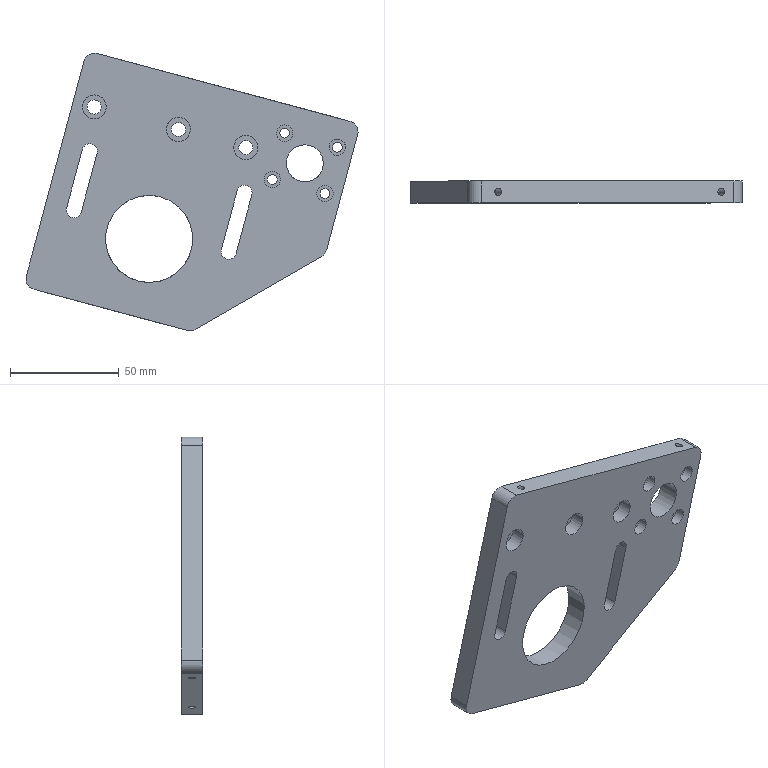Part | 1 solid | 51 faces | box 152.311 x 10 x 127.359 mm | volume 109635 mm3 | cylinder 29 | plane 22 | commonest cylinder face diameters 10 x5 3.3 x4 4.5 x4 7 x4 7.5 x4 6.5 x3
STEP:
#1=CARTESIAN_POINT('',(554.778,-302.903,7.909));
#2=VERTEX_POINT('',#1);
#3=CARTESIAN_POINT('',(554.778,-302.903,-0.5914));
#4=DIRECTION('',(0.,1.,0.));
#5=DIRECTION('',(0.,0.,1.));
#6=AXIS2_PLACEMENT_3D('',#3,#4,#5);
#7=CIRCLE('',#6,8.5);
#8=EDGE_CURVE('',#2,#2,#7,.T.);
#9=ORIENTED_EDGE('',*,*,#8,.T.);
#10=EDGE_LOOP('',(#9));
#11=FACE_BOUND('',#10,.T.);
#12=CARTESIAN_POINT('',(539.857,-302.903,-4.231));
#13=VERTEX_POINT('',#12);
#14=CARTESIAN_POINT('',(539.857,-302.903,-7.981));
#15=DIRECTION('',(0.,1.,0.));
#16=DIRECTION('',(0.,0.,1.));
#17=AXIS2_PLACEMENT_3D('',#14,#15,#16);
#18=CIRCLE('',#17,3.75);
#19=EDGE_CURVE('',#13,#13,#18,.T.);
#20=ORIENTED_EDGE('',*,*,#19,.T.);
#21=EDGE_LOOP('',(#20));
#22=FACE_BOUND('',#21,.T.);
#23=CARTESIAN_POINT('',(527.732,-302.903,12.156));
#24=VERTEX_POINT('',#23);
#25=CARTESIAN_POINT('',(527.732,-302.903,6.656));
#26=DIRECTION('',(0.,1.,0.));
#27=DIRECTION('',(0.,0.,1.));
#28=AXIS2_PLACEMENT_3D('',#25,#26,#27);
#29=CIRCLE('',#28,5.5);
#30=EDGE_CURVE('',#24,#24,#29,.T.);
#31=ORIENTED_EDGE('',*,*,#30,.T.);
#32=EDGE_LOOP('',(#31));
#33=FACE_BOUND('',#32,.T.);
#34=CARTESIAN_POINT('',(530.486,-302.903,-15.015));
#35=VERTEX_POINT('',#34);
#36=CARTESIAN_POINT('',(523.239,-302.903,-42.061));
#37=VERTEX_POINT('',#36);
#38=CARTESIAN_POINT('',(542.399,-302.903,29.442));
#39=DIRECTION('',(-0.2588,0.,-0.9659));
#40=VECTOR('',#39,1000.);
#41=LINE('',#38,#40);
#42=EDGE_CURVE('',#35,#37,#41,.T.);
#43=ORIENTED_EDGE('',*,*,#42,.T.);
#44=CARTESIAN_POINT('',(516.478,-302.903,-40.249));
#45=VERTEX_POINT('',#44);
#46=CARTESIAN_POINT('',(519.859,-302.903,-41.155));
#47=DIRECTION('',(0.,1.,0.));
#48=DIRECTION('',(0.,0.,1.));
#49=AXIS2_PLACEMENT_3D('',#46,#47,#48);
#50=CIRCLE('',#49,3.5);
#51=EDGE_CURVE('',#37,#45,#50,.T.);
#52=ORIENTED_EDGE('',*,*,#51,.T.);
#53=CARTESIAN_POINT('',(523.725,-302.903,-13.203));
#54=VERTEX_POINT('',#53);
#55=CARTESIAN_POINT('',(535.637,-302.903,31.254));
#56=DIRECTION('',(0.2588,0.,0.9659));
#57=VECTOR('',#56,1000.);
#58=LINE('',#55,#57);
#59=EDGE_CURVE('',#45,#54,#58,.T.);
#60=ORIENTED_EDGE('',*,*,#59,.T.);
#61=CARTESIAN_POINT('',(527.106,-302.903,-14.109));
#62=DIRECTION('',(0.,1.,0.));
#63=DIRECTION('',(0.,0.,1.));
#64=AXIS2_PLACEMENT_3D('',#61,#62,#63);
#65=CIRCLE('',#64,3.5);
#66=EDGE_CURVE('',#54,#35,#65,.T.);
#67=ORIENTED_EDGE('',*,*,#66,.T.);
#68=EDGE_LOOP('',(#43,#52,#60,#67));
#69=FACE_BOUND('',#68,.T.);
#70=CARTESIAN_POINT('',(562.508,-302.903,-43.357));
#71=VERTEX_POINT('',#70);
#72=CARTESIAN_POINT('',(564.838,-302.903,-40.321));
#73=VERTEX_POINT('',#72);
#74=CARTESIAN_POINT('',(560.008,-302.903,-39.027));
#75=DIRECTION('',(0.,1.,0.));
#76=DIRECTION('',(0.,0.,1.));
#77=AXIS2_PLACEMENT_3D('',#74,#75,#76);
#78=CIRCLE('',#77,5.);
#79=EDGE_CURVE('',#71,#73,#78,.F.);
#80=ORIENTED_EDGE('',*,*,#79,.T.);
#81=CARTESIAN_POINT('',(579.014,-302.903,12.585));
#82=VERTEX_POINT('',#81);
#83=CARTESIAN_POINT('',(572.802,-302.903,-10.597));
#84=DIRECTION('',(0.2588,0.,0.9659));
#85=VECTOR('',#84,1000.);
#86=LINE('',#83,#85);
#87=EDGE_CURVE('',#73,#82,#86,.T.);
#88=ORIENTED_EDGE('',*,*,#87,.T.);
#89=CARTESIAN_POINT('',(575.478,-302.903,18.709));
#90=VERTEX_POINT('',#89);
#91=CARTESIAN_POINT('',(574.184,-302.903,13.879));
#92=DIRECTION('',(0.,1.,0.));
#93=DIRECTION('',(0.,0.,1.));
#94=AXIS2_PLACEMENT_3D('',#91,#92,#93);
#95=CIRCLE('',#94,5.);
#96=EDGE_CURVE('',#82,#90,#95,.F.);
#97=ORIENTED_EDGE('',*,*,#96,.T.);
#98=CARTESIAN_POINT('',(459.567,-302.903,49.767));
#99=VERTEX_POINT('',#98);
#100=CARTESIAN_POINT('',(344.622,-302.903,80.566));
#101=DIRECTION('',(-0.9659,0.,0.2588));
#102=VECTOR('',#101,1000.);
#103=LINE('',#100,#102);
#104=EDGE_CURVE('',#90,#99,#103,.T.);
#105=ORIENTED_EDGE('',*,*,#104,.T.);
#106=CARTESIAN_POINT('',(453.443,-302.903,46.231));
#107=VERTEX_POINT('',#106);
#108=CARTESIAN_POINT('',(458.273,-302.903,44.937));
#109=DIRECTION('',(0.,1.,0.));
#110=DIRECTION('',(0.,0.,1.));
#111=AXIS2_PLACEMENT_3D('',#108,#109,#110);
#112=CIRCLE('',#111,5.);
#113=EDGE_CURVE('',#99,#107,#112,.F.);
#114=ORIENTED_EDGE('',*,*,#113,.T.);
#115=CARTESIAN_POINT('',(427.044,-302.903,-52.293));
#116=VERTEX_POINT('',#115);
#117=CARTESIAN_POINT('',(425.529,-302.903,-57.947));
#118=DIRECTION('',(-0.2588,0.,-0.9659));
#119=VECTOR('',#118,1000.);
#120=LINE('',#117,#119);
#121=EDGE_CURVE('',#107,#116,#120,.T.);
#122=ORIENTED_EDGE('',*,*,#121,.T.);
#123=CARTESIAN_POINT('',(430.579,-302.903,-58.417));
#124=VERTEX_POINT('',#123);
#125=CARTESIAN_POINT('',(431.874,-302.903,-53.587));
#126=DIRECTION('',(0.,1.,0.));
#127=DIRECTION('',(0.,0.,1.));
#128=AXIS2_PLACEMENT_3D('',#125,#126,#127);
#129=CIRCLE('',#128,5.);
#130=EDGE_CURVE('',#116,#124,#129,.F.);
#131=ORIENTED_EDGE('',*,*,#130,.T.);
#132=CARTESIAN_POINT('',(500.872,-302.903,-77.252));
#133=VERTEX_POINT('',#132);
#134=CARTESIAN_POINT('',(300.037,-302.903,-23.438));
#135=DIRECTION('',(0.9659,0.,-0.2588));
#136=VECTOR('',#135,1000.);
#137=LINE('',#134,#136);
#138=EDGE_CURVE('',#124,#133,#137,.T.);
#139=ORIENTED_EDGE('',*,*,#138,.T.);
#140=CARTESIAN_POINT('',(504.666,-302.903,-76.752));
#141=VERTEX_POINT('',#140);
#142=CARTESIAN_POINT('',(502.166,-302.903,-72.422));
#143=DIRECTION('',(0.,1.,0.));
#144=DIRECTION('',(0.,0.,1.));
#145=AXIS2_PLACEMENT_3D('',#142,#143,#144);
#146=CIRCLE('',#145,5.);
#147=EDGE_CURVE('',#133,#141,#146,.F.);
#148=ORIENTED_EDGE('',*,*,#147,.T.);
#149=CARTESIAN_POINT('',(528.994,-302.903,-62.706));
#150=DIRECTION('',(-0.866,0.,-0.5));
#151=VECTOR('',#150,1000.);
#152=LINE('',#149,#151);
#153=EDGE_CURVE('',#71,#141,#152,.T.);
#154=ORIENTED_EDGE('',*,*,#153,.F.);
#155=EDGE_LOOP('',(#80,#88,#97,#105,#114,#122,#131,#139,#148,#154));
#156=FACE_BOUND('',#155,.T.);
#157=CARTESIAN_POINT('',(452.206,-302.903,-23.027));
#158=VERTEX_POINT('',#157);
#159=CARTESIAN_POINT('',(445.445,-302.903,-21.216));
#160=VERTEX_POINT('',#159);
#161=CARTESIAN_POINT('',(448.826,-302.903,-22.122));
#162=DIRECTION('',(0.,1.,0.));
#163=DIRECTION('',(0.,0.,1.));
#164=AXIS2_PLACEMENT_3D('',#161,#162,#163);
#165=CIRCLE('',#164,3.5);
#166=EDGE_CURVE('',#158,#160,#165,.T.);
#167=ORIENTED_EDGE('',*,*,#166,.T.);
#168=CARTESIAN_POINT('',(452.692,-302.903,5.83));
#169=VERTEX_POINT('',#168);
#170=CARTESIAN_POINT('',(464.604,-302.903,50.287));
#171=DIRECTION('',(0.2588,0.,0.9659));
#172=VECTOR('',#171,1000.);
#173=LINE('',#170,#172);
#174=EDGE_CURVE('',#160,#169,#173,.T.);
#175=ORIENTED_EDGE('',*,*,#174,.T.);
#176=CARTESIAN_POINT('',(459.453,-302.903,4.018));
#177=VERTEX_POINT('',#176);
#178=CARTESIAN_POINT('',(456.072,-302.903,4.924));
#179=DIRECTION('',(0.,1.,0.));
#180=DIRECTION('',(0.,0.,1.));
#181=AXIS2_PLACEMENT_3D('',#178,#179,#180);
#182=CIRCLE('',#181,3.5);
#183=EDGE_CURVE('',#169,#177,#182,.T.);
#184=ORIENTED_EDGE('',*,*,#183,.T.);
#185=CARTESIAN_POINT('',(471.365,-302.903,48.476));
#186=DIRECTION('',(-0.2588,0.,-0.9659));
#187=VECTOR('',#186,1000.);
#188=LINE('',#185,#187);
#189=EDGE_CURVE('',#177,#158,#188,.T.);
#190=ORIENTED_EDGE('',*,*,#189,.T.);
#191=EDGE_LOOP('',(#167,#175,#184,#190));
#192=FACE_BOUND('',#191,.T.);
#193=CARTESIAN_POINT('',(569.699,-302.903,10.549));
#194=VERTEX_POINT('',#193);
#195=CARTESIAN_POINT('',(569.699,-302.903,6.799));
#196=DIRECTION('',(0.,1.,0.));
#197=DIRECTION('',(0.,0.,1.));
#198=AXIS2_PLACEMENT_3D('',#195,#196,#197);
#199=CIRCLE('',#198,3.75);
#200=EDGE_CURVE('',#194,#194,#199,.T.);
#201=ORIENTED_EDGE('',*,*,#200,.T.);
#202=EDGE_LOOP('',(#201));
#203=FACE_BOUND('',#202,.T.);
#204=CARTESIAN_POINT('',(458.185,-302.903,30.791));
#205=VERTEX_POINT('',#204);
#206=CARTESIAN_POINT('',(458.185,-302.903,25.291));
#207=DIRECTION('',(0.,1.,0.));
#208=DIRECTION('',(0.,0.,1.));
#209=AXIS2_PLACEMENT_3D('',#206,#207,#208);
#210=CIRCLE('',#209,5.5);
#211=EDGE_CURVE('',#205,#205,#210,.T.);
#212=ORIENTED_EDGE('',*,*,#211,.T.);
#213=EDGE_LOOP('',(#212));
#214=FACE_BOUND('',#213,.T.);
#215=CARTESIAN_POINT('',(496.822,-302.903,20.438));
#216=VERTEX_POINT('',#215);
#217=CARTESIAN_POINT('',(496.822,-302.903,14.938));
#218=DIRECTION('',(0.,1.,0.));
#219=DIRECTION('',(0.,0.,1.));
#220=AXIS2_PLACEMENT_3D('',#217,#218,#219);
#221=CIRCLE('',#220,5.5);
#222=EDGE_CURVE('',#216,#216,#221,.T.);
#223=ORIENTED_EDGE('',*,*,#222,.T.);
#224=EDGE_LOOP('',(#223));
#225=FACE_BOUND('',#224,.T.);
#226=CARTESIAN_POINT('',(564.005,-302.903,-10.702));
#227=VERTEX_POINT('',#226);
#228=CARTESIAN_POINT('',(564.005,-302.903,-14.452));
#229=DIRECTION('',(0.,1.,0.));
#230=DIRECTION('',(0.,0.,1.));
#231=AXIS2_PLACEMENT_3D('',#228,#229,#230);
#232=CIRCLE('',#231,3.75);
#233=EDGE_CURVE('',#227,#227,#232,.T.);
#234=ORIENTED_EDGE('',*,*,#233,.T.);
#235=EDGE_LOOP('',(#234));
#236=FACE_BOUND('',#235,.T.);
#237=CARTESIAN_POINT('',(545.551,-302.903,17.019));
#238=VERTEX_POINT('',#237);
#239=CARTESIAN_POINT('',(545.551,-302.903,13.269));
#240=DIRECTION('',(0.,1.,0.));
#241=DIRECTION('',(0.,0.,1.));
#242=AXIS2_PLACEMENT_3D('',#239,#240,#241);
#243=CIRCLE('',#242,3.75);
#244=EDGE_CURVE('',#238,#238,#243,.T.);
#245=ORIENTED_EDGE('',*,*,#244,.T.);
#246=EDGE_LOOP('',(#245));
#247=FACE_BOUND('',#246,.T.);
#248=CARTESIAN_POINT('',(483.367,-302.903,-15.279));
#249=VERTEX_POINT('',#248);
#250=CARTESIAN_POINT('',(483.367,-302.903,-35.279));
#251=DIRECTION('',(0.,1.,0.));
#252=DIRECTION('',(0.,0.,1.));
#253=AXIS2_PLACEMENT_3D('',#250,#251,#252);
#254=CIRCLE('',#253,20.);
#255=EDGE_CURVE('',#249,#249,#254,.T.);
#256=ORIENTED_EDGE('',*,*,#255,.T.);
#257=EDGE_LOOP('',(#256));
#258=FACE_BOUND('',#257,.T.);
#259=CARTESIAN_POINT('',(599.269,-302.903,14.204));
#260=DIRECTION('',(0.,1.,0.));
#261=DIRECTION('',(0.7196,0.,-0.6944));
#262=AXIS2_PLACEMENT_3D('',#259,#260,#261);
#263=PLANE('',#262);
#264=ADVANCED_FACE('',(#11,#22,#33,#69,#156,#192,#203,#214,#225,#236,#247,#258),#263,.F.);
#265=CARTESIAN_POINT('',(492.717,-297.903,-64.714));
#266=VERTEX_POINT('',#265);
#267=CARTESIAN_POINT('',(491.123,-297.903,-64.287));
#268=DIRECTION('',(0.2588,0.,0.9659));
#269=DIRECTION('',(0.9659,0.,-0.2588));
#270=AXIS2_PLACEMENT_3D('',#267,#268,#269);
#271=CIRCLE('',#270,1.65);
#272=EDGE_CURVE('',#266,#266,#271,.T.);
#273=ORIENTED_EDGE('',*,*,#272,.T.);
#274=EDGE_LOOP('',(#273));
#275=FACE_BOUND('',#274,.T.);
#276=CARTESIAN_POINT('',(490.129,-297.903,-74.373));
#277=VERTEX_POINT('',#276);
#278=CARTESIAN_POINT('',(488.535,-297.903,-73.946));
#279=DIRECTION('',(0.2588,0.,0.9659));
#280=DIRECTION('',(0.9659,0.,-0.2588));
#281=AXIS2_PLACEMENT_3D('',#278,#279,#280);
#282=CIRCLE('',#281,1.65);
#283=EDGE_CURVE('',#277,#277,#282,.T.);
#284=ORIENTED_EDGE('',*,*,#283,.F.);
#285=EDGE_LOOP('',(#284));
#286=FACE_BOUND('',#285,.T.);
#287=CARTESIAN_POINT('',(489.829,-297.903,-69.116));
#288=DIRECTION('',(-0.2588,0.,-0.9659));
#289=DIRECTION('',(0.,1.,0.));
#290=AXIS2_PLACEMENT_3D('',#287,#288,#289);
#291=CYLINDRICAL_SURFACE('',#290,1.65);
#292=ADVANCED_FACE('',(#275,#286),#291,.F.);
#293=ORIENTED_EDGE('',*,*,#272,.F.);
#294=EDGE_LOOP('',(#293));
#295=FACE_BOUND('',#294,.T.);
#296=CARTESIAN_POINT('',(442.827,-297.903,-51.346));
#297=DIRECTION('',(0.2588,0.,0.9659));
#298=DIRECTION('',(-0.9659,0.,0.2588));
#299=AXIS2_PLACEMENT_3D('',#296,#297,#298);
#300=PLANE('',#299);
#301=ADVANCED_FACE('',(#295),#300,.F.);
#302=CARTESIAN_POINT('',(568.302,-298.98,10.279));
#303=VERTEX_POINT('',#302);
#304=CARTESIAN_POINT('',(568.669,-298.403,10.405));
#305=VERTEX_POINT('',#304);
#306=CARTESIAN_POINT('',(568.302,-298.98,10.279));
#307=CARTESIAN_POINT('',(568.462,-298.819,10.343));
#308=CARTESIAN_POINT('',(568.591,-298.624,10.382));
#309=CARTESIAN_POINT('',(568.669,-298.403,10.405));
#310=B_SPLINE_CURVE_WITH_KNOTS('',3,(#306,#307,#308,#309),.UNSPECIFIED.,.F.,.F.,(4,4),(0.,0.0006972),.UNSPECIFIED.);
#311=EDGE_CURVE('',#303,#305,#310,.T.);
#312=ORIENTED_EDGE('',*,*,#311,.F.);
#313=CARTESIAN_POINT('',(568.613,-298.403,10.195));
#314=VERTEX_POINT('',#313);
#315=CARTESIAN_POINT('',(567.095,-297.903,10.602));
#316=DIRECTION('',(-0.2588,0.,-0.9659));
#317=DIRECTION('',(-0.9659,0.,0.2588));
#318=AXIS2_PLACEMENT_3D('',#315,#316,#317);
#319=CIRCLE('',#318,1.65);
#320=EDGE_CURVE('',#303,#314,#319,.T.);
#321=ORIENTED_EDGE('',*,*,#320,.T.);
#322=CARTESIAN_POINT('',(569.907,-298.403,15.025));
#323=DIRECTION('',(-0.2588,0.,-0.9659));
#324=VECTOR('',#323,1000.);
#325=LINE('',#322,#324);
#326=EDGE_CURVE('',#305,#314,#325,.T.);
#327=ORIENTED_EDGE('',*,*,#326,.F.);
#328=EDGE_LOOP('',(#312,#321,#327));
#329=FACE_BOUND('',#328,.T.);
#330=CARTESIAN_POINT('',(568.089,-297.903,20.689));
#331=VERTEX_POINT('',#330);
#332=CARTESIAN_POINT('',(569.683,-297.903,20.261));
#333=DIRECTION('',(-0.2588,0.,-0.9659));
#334=DIRECTION('',(-0.9659,0.,0.2588));
#335=AXIS2_PLACEMENT_3D('',#332,#333,#334);
#336=CIRCLE('',#335,1.65);
#337=EDGE_CURVE('',#331,#331,#336,.T.);
#338=ORIENTED_EDGE('',*,*,#337,.F.);
#339=EDGE_LOOP('',(#338));
#340=FACE_BOUND('',#339,.T.);
#341=CARTESIAN_POINT('',(568.389,-297.903,15.432));
#342=DIRECTION('',(0.2588,0.,0.9659));
#343=DIRECTION('',(0.,1.,0.));
#344=AXIS2_PLACEMENT_3D('',#341,#342,#343);
#345=CYLINDRICAL_SURFACE('',#344,1.65);
#346=ADVANCED_FACE('',(#329,#340),#345,.F.);
#347=ORIENTED_EDGE('',*,*,#320,.F.);
#348=CARTESIAN_POINT('',(568.302,-298.403,10.279));
#349=VERTEX_POINT('',#348);
#350=CARTESIAN_POINT('',(568.302,-302.903,10.279));
#351=DIRECTION('',(0.,-1.,0.));
#352=VECTOR('',#351,1000.);
#353=LINE('',#350,#352);
#354=EDGE_CURVE('',#349,#303,#353,.T.);
#355=ORIENTED_EDGE('',*,*,#354,.F.);
#356=CARTESIAN_POINT('',(570.475,-298.403,9.696));
#357=DIRECTION('',(-0.9659,0.,0.2588));
#358=VECTOR('',#357,1000.);
#359=LINE('',#356,#358);
#360=EDGE_CURVE('',#314,#349,#359,.T.);
#361=ORIENTED_EDGE('',*,*,#360,.F.);
#362=EDGE_LOOP('',(#347,#355,#361));
#363=FACE_BOUND('',#362,.T.);
#364=CARTESIAN_POINT('',(466.638,-297.903,37.519));
#365=DIRECTION('',(-0.2588,0.,-0.9659));
#366=DIRECTION('',(-0.9659,0.,0.2588));
#367=AXIS2_PLACEMENT_3D('',#364,#365,#366);
#368=PLANE('',#367);
#369=ADVANCED_FACE('',(#363),#368,.F.);
#370=CARTESIAN_POINT('',(442.489,-297.903,-51.255));
#371=VERTEX_POINT('',#370);
#372=CARTESIAN_POINT('',(440.895,-297.903,-50.828));
#373=DIRECTION('',(0.2588,0.,0.9659));
#374=DIRECTION('',(0.9659,0.,-0.2588));
#375=AXIS2_PLACEMENT_3D('',#372,#373,#374);
#376=CIRCLE('',#375,1.65);
#377=EDGE_CURVE('',#371,#371,#376,.T.);
#378=ORIENTED_EDGE('',*,*,#377,.T.);
#379=EDGE_LOOP('',(#378));
#380=FACE_BOUND('',#379,.T.);
#381=CARTESIAN_POINT('',(436.713,-297.903,-60.06));
#382=VERTEX_POINT('',#381);
#383=CARTESIAN_POINT('',(438.307,-297.903,-60.487));
#384=DIRECTION('',(0.2588,0.,0.9659));
#385=DIRECTION('',(-0.9659,0.,0.2588));
#386=AXIS2_PLACEMENT_3D('',#383,#384,#385);
#387=CIRCLE('',#386,1.65);
#388=EDGE_CURVE('',#382,#382,#387,.T.);
#389=ORIENTED_EDGE('',*,*,#388,.F.);
#390=EDGE_LOOP('',(#389));
#391=FACE_BOUND('',#390,.T.);
#392=CARTESIAN_POINT('',(466.,-297.903,42.867));
#393=DIRECTION('',(0.2588,0.,0.9659));
#394=DIRECTION('',(0.,1.,0.));
#395=AXIS2_PLACEMENT_3D('',#392,#393,#394);
#396=CYLINDRICAL_SURFACE('',#395,1.65);
#397=ADVANCED_FACE('',(#380,#391),#396,.F.);
#398=ORIENTED_EDGE('',*,*,#377,.F.);
#399=EDGE_LOOP('',(#398));
#400=FACE_BOUND('',#399,.T.);
#401=CARTESIAN_POINT('',(442.827,-297.903,-51.346));
#402=DIRECTION('',(0.2588,0.,0.9659));
#403=DIRECTION('',(-0.9659,0.,0.2588));
#404=AXIS2_PLACEMENT_3D('',#401,#402,#403);
#405=PLANE('',#404);
#406=ADVANCED_FACE('',(#400),#405,.F.);
#407=CARTESIAN_POINT('',(463.113,-297.903,38.464));
#408=VERTEX_POINT('',#407);
#409=CARTESIAN_POINT('',(464.706,-297.903,38.037));
#410=DIRECTION('',(-0.2588,0.,-0.9659));
#411=DIRECTION('',(-0.9659,0.,0.2588));
#412=AXIS2_PLACEMENT_3D('',#409,#410,#411);
#413=CIRCLE('',#412,1.65);
#414=EDGE_CURVE('',#408,#408,#413,.T.);
#415=ORIENTED_EDGE('',*,*,#414,.T.);
#416=EDGE_LOOP('',(#415));
#417=FACE_BOUND('',#416,.T.);
#418=CARTESIAN_POINT('',(468.888,-297.903,47.269));
#419=VERTEX_POINT('',#418);
#420=CARTESIAN_POINT('',(467.295,-297.903,47.696));
#421=DIRECTION('',(-0.2588,0.,-0.9659));
#422=DIRECTION('',(0.9659,0.,-0.2588));
#423=AXIS2_PLACEMENT_3D('',#420,#421,#422);
#424=CIRCLE('',#423,1.65);
#425=EDGE_CURVE('',#419,#419,#424,.T.);
#426=ORIENTED_EDGE('',*,*,#425,.F.);
#427=EDGE_LOOP('',(#426));
#428=FACE_BOUND('',#427,.T.);
#429=CARTESIAN_POINT('',(466.,-297.903,42.867));
#430=DIRECTION('',(0.2588,0.,0.9659));
#431=DIRECTION('',(0.,1.,0.));
#432=AXIS2_PLACEMENT_3D('',#429,#430,#431);
#433=CYLINDRICAL_SURFACE('',#432,1.65);
#434=ADVANCED_FACE('',(#417,#428),#433,.F.);
#435=ORIENTED_EDGE('',*,*,#414,.F.);
#436=EDGE_LOOP('',(#435));
#437=FACE_BOUND('',#436,.T.);
#438=CARTESIAN_POINT('',(466.638,-297.903,37.519));
#439=DIRECTION('',(-0.2588,0.,-0.9659));
#440=DIRECTION('',(-0.9659,0.,0.2588));
#441=AXIS2_PLACEMENT_3D('',#438,#439,#440);
#442=PLANE('',#441);
#443=ADVANCED_FACE('',(#437),#442,.F.);
#444=CARTESIAN_POINT('',(564.005,-298.403,-10.702));
#445=VERTEX_POINT('',#444);
#446=CARTESIAN_POINT('',(564.005,-298.403,-14.452));
#447=DIRECTION('',(0.,-1.,0.));
#448=DIRECTION('',(0.,0.,1.));
#449=AXIS2_PLACEMENT_3D('',#446,#447,#448);
#450=CIRCLE('',#449,3.75);
#451=EDGE_CURVE('',#445,#445,#450,.T.);
#452=ORIENTED_EDGE('',*,*,#451,.F.);
#453=EDGE_LOOP('',(#452));
#454=FACE_BOUND('',#453,.T.);
#455=ORIENTED_EDGE('',*,*,#233,.F.);
#456=EDGE_LOOP('',(#455));
#457=FACE_BOUND('',#456,.T.);
#458=CARTESIAN_POINT('',(564.005,-302.903,-14.452));
#459=DIRECTION('',(0.,1.,0.));
#460=DIRECTION('',(-0.9659,0.,0.2588));
#461=AXIS2_PLACEMENT_3D('',#458,#459,#460);
#462=CYLINDRICAL_SURFACE('',#461,3.75);
#463=ADVANCED_FACE('',(#454,#457),#462,.F.);
#464=ORIENTED_EDGE('',*,*,#451,.T.);
#465=EDGE_LOOP('',(#464));
#466=FACE_BOUND('',#465,.T.);
#467=CARTESIAN_POINT('',(564.005,-298.403,-12.202));
#468=VERTEX_POINT('',#467);
#469=CARTESIAN_POINT('',(564.005,-298.403,-14.452));
#470=DIRECTION('',(0.,-1.,0.));
#471=DIRECTION('',(0.,0.,1.));
#472=AXIS2_PLACEMENT_3D('',#469,#470,#471);
#473=CIRCLE('',#472,2.25);
#474=EDGE_CURVE('',#468,#468,#473,.T.);
#475=ORIENTED_EDGE('',*,*,#474,.F.);
#476=EDGE_LOOP('',(#475));
#477=FACE_BOUND('',#476,.T.);
#478=CARTESIAN_POINT('',(569.699,-298.403,6.799));
#479=DIRECTION('',(0.,1.,0.));
#480=DIRECTION('',(-0.9659,0.,0.2588));
#481=AXIS2_PLACEMENT_3D('',#478,#479,#480);
#482=PLANE('',#481);
#483=ADVANCED_FACE('',(#466,#477),#482,.F.);
#484=CARTESIAN_POINT('',(564.587,-292.903,-12.278));
#485=VERTEX_POINT('',#484);
#486=CARTESIAN_POINT('',(564.005,-292.903,-14.452));
#487=DIRECTION('',(0.,1.,0.));
#488=DIRECTION('',(0.2588,0.,0.9659));
#489=AXIS2_PLACEMENT_3D('',#486,#487,#488);
#490=CIRCLE('',#489,2.25);
#491=EDGE_CURVE('',#485,#485,#490,.T.);
#492=ORIENTED_EDGE('',*,*,#491,.T.);
#493=EDGE_LOOP('',(#492));
#494=FACE_BOUND('',#493,.T.);
#495=ORIENTED_EDGE('',*,*,#474,.T.);
#496=EDGE_LOOP('',(#495));
#497=FACE_BOUND('',#496,.T.);
#498=CARTESIAN_POINT('',(564.005,-232.903,-14.452));
#499=DIRECTION('',(0.,1.,0.));
#500=DIRECTION('',(-0.9659,0.,0.2588));
#501=AXIS2_PLACEMENT_3D('',#498,#499,#500);
#502=CYLINDRICAL_SURFACE('',#501,2.25);
#503=ADVANCED_FACE('',(#494,#497),#502,.F.);
#504=CARTESIAN_POINT('',(569.699,-298.403,6.799));
#505=DIRECTION('',(0.,1.,0.));
#506=DIRECTION('',(-0.9659,0.,0.2588));
#507=AXIS2_PLACEMENT_3D('',#504,#505,#506);
#508=CIRCLE('',#507,3.75);
#509=EDGE_CURVE('',#305,#349,#508,.T.);
#510=ORIENTED_EDGE('',*,*,#509,.T.);
#511=ORIENTED_EDGE('',*,*,#354,.T.);
#512=ORIENTED_EDGE('',*,*,#311,.T.);
#513=EDGE_LOOP('',(#510,#511,#512));
#514=FACE_BOUND('',#513,.T.);
#515=ORIENTED_EDGE('',*,*,#200,.F.);
#516=EDGE_LOOP('',(#515));
#517=FACE_BOUND('',#516,.T.);
#518=CARTESIAN_POINT('',(569.699,-302.903,6.799));
#519=DIRECTION('',(0.,1.,0.));
#520=DIRECTION('',(-0.9659,0.,0.2588));
#521=AXIS2_PLACEMENT_3D('',#518,#519,#520);
#522=CYLINDRICAL_SURFACE('',#521,3.75);
#523=ADVANCED_FACE('',(#514,#517),#522,.F.);
#524=ORIENTED_EDGE('',*,*,#326,.T.);
#525=ORIENTED_EDGE('',*,*,#360,.T.);
#526=ORIENTED_EDGE('',*,*,#509,.F.);
#527=EDGE_LOOP('',(#524,#525,#526));
#528=FACE_BOUND('',#527,.T.);
#529=CARTESIAN_POINT('',(567.525,-298.403,7.381));
#530=VERTEX_POINT('',#529);
#531=CARTESIAN_POINT('',(569.699,-298.403,6.799));
#532=DIRECTION('',(0.,1.,0.));
#533=DIRECTION('',(-0.9659,0.,0.2588));
#534=AXIS2_PLACEMENT_3D('',#531,#532,#533);
#535=CIRCLE('',#534,2.25);
#536=EDGE_CURVE('',#530,#530,#535,.T.);
#537=ORIENTED_EDGE('',*,*,#536,.T.);
#538=EDGE_LOOP('',(#537));
#539=FACE_BOUND('',#538,.T.);
#540=CARTESIAN_POINT('',(569.699,-298.403,6.799));
#541=DIRECTION('',(0.,1.,0.));
#542=DIRECTION('',(-0.9659,0.,0.2588));
#543=AXIS2_PLACEMENT_3D('',#540,#541,#542);
#544=PLANE('',#543);
#545=ADVANCED_FACE('',(#528,#539),#544,.F.);
#546=CARTESIAN_POINT('',(570.281,-292.903,8.972));
#547=VERTEX_POINT('',#546);
#548=CARTESIAN_POINT('',(569.699,-292.903,6.799));
#549=DIRECTION('',(0.,-1.,0.));
#550=DIRECTION('',(0.2588,0.,0.9659));
#551=AXIS2_PLACEMENT_3D('',#548,#549,#550);
#552=CIRCLE('',#551,2.25);
#553=EDGE_CURVE('',#547,#547,#552,.T.);
#554=ORIENTED_EDGE('',*,*,#553,.F.);
#555=EDGE_LOOP('',(#554));
#556=FACE_BOUND('',#555,.T.);
#557=ORIENTED_EDGE('',*,*,#536,.F.);
#558=EDGE_LOOP('',(#557));
#559=FACE_BOUND('',#558,.T.);
#560=CARTESIAN_POINT('',(569.699,-232.903,6.799));
#561=DIRECTION('',(0.,1.,0.));
#562=DIRECTION('',(-0.9659,0.,0.2588));
#563=AXIS2_PLACEMENT_3D('',#560,#561,#562);
#564=CYLINDRICAL_SURFACE('',#563,2.25);
#565=ADVANCED_FACE('',(#556,#559),#564,.F.);
#566=CARTESIAN_POINT('',(539.857,-298.403,-4.231));
#567=VERTEX_POINT('',#566);
#568=CARTESIAN_POINT('',(539.857,-298.403,-7.981));
#569=DIRECTION('',(0.,1.,0.));
#570=DIRECTION('',(0.,0.,1.));
#571=AXIS2_PLACEMENT_3D('',#568,#569,#570);
#572=CIRCLE('',#571,3.75);
#573=EDGE_CURVE('',#567,#567,#572,.T.);
#574=ORIENTED_EDGE('',*,*,#573,.T.);
#575=EDGE_LOOP('',(#574));
#576=FACE_BOUND('',#575,.T.);
#577=ORIENTED_EDGE('',*,*,#19,.F.);
#578=EDGE_LOOP('',(#577));
#579=FACE_BOUND('',#578,.T.);
#580=CARTESIAN_POINT('',(539.857,-302.903,-7.981));
#581=DIRECTION('',(0.,1.,0.));
#582=DIRECTION('',(-0.9659,0.,0.2588));
#583=AXIS2_PLACEMENT_3D('',#580,#581,#582);
#584=CYLINDRICAL_SURFACE('',#583,3.75);
#585=ADVANCED_FACE('',(#576,#579),#584,.F.);
#586=ORIENTED_EDGE('',*,*,#573,.F.);
#587=EDGE_LOOP('',(#586));
#588=FACE_BOUND('',#587,.T.);
#589=CARTESIAN_POINT('',(539.857,-298.403,-5.731));
#590=VERTEX_POINT('',#589);
#591=CARTESIAN_POINT('',(539.857,-298.403,-7.981));
#592=DIRECTION('',(0.,1.,0.));
#593=DIRECTION('',(0.,0.,1.));
#594=AXIS2_PLACEMENT_3D('',#591,#592,#593);
#595=CIRCLE('',#594,2.25);
#596=EDGE_CURVE('',#590,#590,#595,.T.);
#597=ORIENTED_EDGE('',*,*,#596,.T.);
#598=EDGE_LOOP('',(#597));
#599=FACE_BOUND('',#598,.T.);
#600=CARTESIAN_POINT('',(569.699,-298.403,6.799));
#601=DIRECTION('',(0.,1.,0.));
#602=DIRECTION('',(-0.9659,0.,0.2588));
#603=AXIS2_PLACEMENT_3D('',#600,#601,#602);
#604=PLANE('',#603);
#605=ADVANCED_FACE('',(#588,#599),#604,.F.);
#606=CARTESIAN_POINT('',(540.439,-292.903,-5.808));
#607=VERTEX_POINT('',#606);
#608=CARTESIAN_POINT('',(539.857,-292.903,-7.981));
#609=DIRECTION('',(0.,-1.,0.));
#610=DIRECTION('',(0.2588,0.,0.9659));
#611=AXIS2_PLACEMENT_3D('',#608,#609,#610);
#612=CIRCLE('',#611,2.25);
#613=EDGE_CURVE('',#607,#607,#612,.T.);
#614=ORIENTED_EDGE('',*,*,#613,.F.);
#615=EDGE_LOOP('',(#614));
#616=FACE_BOUND('',#615,.T.);
#617=ORIENTED_EDGE('',*,*,#596,.F.);
#618=EDGE_LOOP('',(#617));
#619=FACE_BOUND('',#618,.T.);
#620=CARTESIAN_POINT('',(539.857,-232.903,-7.981));
#621=DIRECTION('',(0.,1.,0.));
#622=DIRECTION('',(-0.9659,0.,0.2588));
#623=AXIS2_PLACEMENT_3D('',#620,#621,#622);
#624=CYLINDRICAL_SURFACE('',#623,2.25);
#625=ADVANCED_FACE('',(#616,#619),#624,.F.);
#626=CARTESIAN_POINT('',(545.551,-298.403,17.019));
#627=VERTEX_POINT('',#626);
#628=CARTESIAN_POINT('',(545.551,-298.403,13.269));
#629=DIRECTION('',(0.,-1.,0.));
#630=DIRECTION('',(0.,0.,1.));
#631=AXIS2_PLACEMENT_3D('',#628,#629,#630);
#632=CIRCLE('',#631,3.75);
#633=EDGE_CURVE('',#627,#627,#632,.T.);
#634=ORIENTED_EDGE('',*,*,#633,.F.);
#635=EDGE_LOOP('',(#634));
#636=FACE_BOUND('',#635,.T.);
#637=ORIENTED_EDGE('',*,*,#244,.F.);
#638=EDGE_LOOP('',(#637));
#639=FACE_BOUND('',#638,.T.);
#640=CARTESIAN_POINT('',(545.551,-302.903,13.269));
#641=DIRECTION('',(0.,1.,0.));
#642=DIRECTION('',(-0.9659,0.,0.2588));
#643=AXIS2_PLACEMENT_3D('',#640,#641,#642);
#644=CYLINDRICAL_SURFACE('',#643,3.75);
#645=ADVANCED_FACE('',(#636,#639),#644,.F.);
#646=ORIENTED_EDGE('',*,*,#633,.T.);
#647=EDGE_LOOP('',(#646));
#648=FACE_BOUND('',#647,.T.);
#649=CARTESIAN_POINT('',(545.551,-298.403,15.519));
#650=VERTEX_POINT('',#649);
#651=CARTESIAN_POINT('',(545.551,-298.403,13.269));
#652=DIRECTION('',(0.,-1.,0.));
#653=DIRECTION('',(0.,0.,1.));
#654=AXIS2_PLACEMENT_3D('',#651,#652,#653);
#655=CIRCLE('',#654,2.25);
#656=EDGE_CURVE('',#650,#650,#655,.T.);
#657=ORIENTED_EDGE('',*,*,#656,.F.);
#658=EDGE_LOOP('',(#657));
#659=FACE_BOUND('',#658,.T.);
#660=CARTESIAN_POINT('',(569.699,-298.403,6.799));
#661=DIRECTION('',(0.,1.,0.));
#662=DIRECTION('',(-0.9659,0.,0.2588));
#663=AXIS2_PLACEMENT_3D('',#660,#661,#662);
#664=PLANE('',#663);
#665=ADVANCED_FACE('',(#648,#659),#664,.F.);
#666=CARTESIAN_POINT('',(546.133,-292.903,15.442));
#667=VERTEX_POINT('',#666);
#668=CARTESIAN_POINT('',(545.551,-292.903,13.269));
#669=DIRECTION('',(0.,-1.,0.));
#670=DIRECTION('',(0.2588,0.,0.9659));
#671=AXIS2_PLACEMENT_3D('',#668,#669,#670);
#672=CIRCLE('',#671,2.25);
#673=EDGE_CURVE('',#667,#667,#672,.T.);
#674=ORIENTED_EDGE('',*,*,#673,.F.);
#675=EDGE_LOOP('',(#674));
#676=FACE_BOUND('',#675,.T.);
#677=ORIENTED_EDGE('',*,*,#656,.T.);
#678=EDGE_LOOP('',(#677));
#679=FACE_BOUND('',#678,.T.);
#680=CARTESIAN_POINT('',(545.551,-232.903,13.269));
#681=DIRECTION('',(0.,1.,0.));
#682=DIRECTION('',(-0.9659,0.,0.2588));
#683=AXIS2_PLACEMENT_3D('',#680,#681,#682);
#684=CYLINDRICAL_SURFACE('',#683,2.25);
#685=ADVANCED_FACE('',(#676,#679),#684,.F.);
#686=ORIENTED_EDGE('',*,*,#113,.F.);
#687=CARTESIAN_POINT('',(459.567,-292.903,49.767));
#688=VERTEX_POINT('',#687);
#689=CARTESIAN_POINT('',(459.567,-302.903,49.767));
#690=DIRECTION('',(0.,-1.,0.));
#691=VECTOR('',#690,1000.);
#692=LINE('',#689,#691);
#693=EDGE_CURVE('',#688,#99,#692,.T.);
#694=ORIENTED_EDGE('',*,*,#693,.F.);
#695=CARTESIAN_POINT('',(453.443,-292.903,46.231));
#696=VERTEX_POINT('',#695);
#697=CARTESIAN_POINT('',(458.273,-292.903,44.937));
#698=DIRECTION('',(0.,1.,0.));
#699=DIRECTION('',(0.2588,0.,0.9659));
#700=AXIS2_PLACEMENT_3D('',#697,#698,#699);
#701=CIRCLE('',#700,5.);
#702=EDGE_CURVE('',#696,#688,#701,.T.);
#703=ORIENTED_EDGE('',*,*,#702,.F.);
#704=CARTESIAN_POINT('',(453.443,-292.903,46.231));
#705=DIRECTION('',(0.,1.,0.));
#706=VECTOR('',#705,1000.);
#707=LINE('',#704,#706);
#708=EDGE_CURVE('',#107,#696,#707,.T.);
#709=ORIENTED_EDGE('',*,*,#708,.F.);
#710=EDGE_LOOP('',(#686,#694,#703,#709));
#711=FACE_BOUND('',#710,.T.);
#712=CARTESIAN_POINT('',(458.273,-270.003,44.937));
#713=DIRECTION('',(0.,1.,0.));
#714=DIRECTION('',(-0.9659,0.,0.2588));
#715=AXIS2_PLACEMENT_3D('',#712,#713,#714);
#716=CYLINDRICAL_SURFACE('',#715,5.);
#717=ADVANCED_FACE('',(#711),#716,.T.);
#718=ORIENTED_EDGE('',*,*,#130,.F.);
#719=CARTESIAN_POINT('',(427.044,-292.903,-52.293));
#720=VERTEX_POINT('',#719);
#721=CARTESIAN_POINT('',(427.044,-302.903,-52.293));
#722=DIRECTION('',(0.,-1.,0.));
#723=VECTOR('',#722,1000.);
#724=LINE('',#721,#723);
#725=EDGE_CURVE('',#720,#116,#724,.T.);
#726=ORIENTED_EDGE('',*,*,#725,.F.);
#727=CARTESIAN_POINT('',(430.579,-292.903,-58.417));
#728=VERTEX_POINT('',#727);
#729=CARTESIAN_POINT('',(431.874,-292.903,-53.587));
#730=DIRECTION('',(0.,1.,0.));
#731=DIRECTION('',(0.2588,0.,0.9659));
#732=AXIS2_PLACEMENT_3D('',#729,#730,#731);
#733=CIRCLE('',#732,5.);
#734=EDGE_CURVE('',#728,#720,#733,.T.);
#735=ORIENTED_EDGE('',*,*,#734,.F.);
#736=CARTESIAN_POINT('',(430.579,-292.903,-58.417));
#737=DIRECTION('',(0.,1.,0.));
#738=VECTOR('',#737,1000.);
#739=LINE('',#736,#738);
#740=EDGE_CURVE('',#124,#728,#739,.T.);
#741=ORIENTED_EDGE('',*,*,#740,.F.);
#742=EDGE_LOOP('',(#718,#726,#735,#741));
#743=FACE_BOUND('',#742,.T.);
#744=CARTESIAN_POINT('',(431.874,-270.003,-53.587));
#745=DIRECTION('',(0.,-1.,0.));
#746=DIRECTION('',(0.9659,0.,-0.2588));
#747=AXIS2_PLACEMENT_3D('',#744,#745,#746);
#748=CYLINDRICAL_SURFACE('',#747,5.);
#749=ADVANCED_FACE('',(#743),#748,.T.);
#750=ORIENTED_EDGE('',*,*,#79,.F.);
#751=CARTESIAN_POINT('',(562.508,-292.903,-43.357));
#752=VERTEX_POINT('',#751);
#753=CARTESIAN_POINT('',(562.508,-318.403,-43.357));
#754=DIRECTION('',(0.,-1.,0.));
#755=VECTOR('',#754,1000.);
#756=LINE('',#753,#755);
#757=EDGE_CURVE('',#752,#71,#756,.T.);
#758=ORIENTED_EDGE('',*,*,#757,.F.);
#759=CARTESIAN_POINT('',(564.838,-292.903,-40.321));
#760=VERTEX_POINT('',#759);
#761=CARTESIAN_POINT('',(560.008,-292.903,-39.027));
#762=DIRECTION('',(0.,1.,0.));
#763=DIRECTION('',(0.2588,0.,0.9659));
#764=AXIS2_PLACEMENT_3D('',#761,#762,#763);
#765=CIRCLE('',#764,5.);
#766=EDGE_CURVE('',#760,#752,#765,.T.);
#767=ORIENTED_EDGE('',*,*,#766,.F.);
#768=CARTESIAN_POINT('',(564.838,-279.903,-40.321));
#769=DIRECTION('',(0.,1.,0.));
#770=VECTOR('',#769,1000.);
#771=LINE('',#768,#770);
#772=EDGE_CURVE('',#73,#760,#771,.T.);
#773=ORIENTED_EDGE('',*,*,#772,.F.);
#774=EDGE_LOOP('',(#750,#758,#767,#773));
#775=FACE_BOUND('',#774,.T.);
#776=CARTESIAN_POINT('',(560.008,-279.903,-39.027));
#777=DIRECTION('',(0.,-1.,0.));
#778=DIRECTION('',(0.2588,0.,0.9659));
#779=AXIS2_PLACEMENT_3D('',#776,#777,#778);
#780=CYLINDRICAL_SURFACE('',#779,5.);
#781=ADVANCED_FACE('',(#775),#780,.T.);
#782=ORIENTED_EDGE('',*,*,#147,.F.);
#783=CARTESIAN_POINT('',(500.872,-292.903,-77.252));
#784=VERTEX_POINT('',#783);
#785=CARTESIAN_POINT('',(500.872,-293.653,-77.252));
#786=DIRECTION('',(0.,-1.,0.));
#787=VECTOR('',#786,1000.);
#788=LINE('',#785,#787);
#789=EDGE_CURVE('',#784,#133,#788,.T.);
#790=ORIENTED_EDGE('',*,*,#789,.F.);
#791=CARTESIAN_POINT('',(504.666,-292.903,-76.752));
#792=VERTEX_POINT('',#791);
#793=CARTESIAN_POINT('',(502.166,-292.903,-72.422));
#794=DIRECTION('',(0.,1.,0.));
#795=DIRECTION('',(0.2588,0.,0.9659));
#796=AXIS2_PLACEMENT_3D('',#793,#794,#795);
#797=CIRCLE('',#796,5.);
#798=EDGE_CURVE('',#792,#784,#797,.T.);
#799=ORIENTED_EDGE('',*,*,#798,.F.);
#800=CARTESIAN_POINT('',(504.666,-318.403,-76.752));
#801=DIRECTION('',(0.,1.,0.));
#802=VECTOR('',#801,1000.);
#803=LINE('',#800,#802);
#804=EDGE_CURVE('',#141,#792,#803,.T.);
#805=ORIENTED_EDGE('',*,*,#804,.F.);
#806=EDGE_LOOP('',(#782,#790,#799,#805));
#807=FACE_BOUND('',#806,.T.);
#808=CARTESIAN_POINT('',(502.166,-293.653,-72.422));
#809=DIRECTION('',(0.,1.,0.));
#810=DIRECTION('',(-0.9659,0.,0.2588));
#811=AXIS2_PLACEMENT_3D('',#808,#809,#810);
#812=CYLINDRICAL_SURFACE('',#811,5.);
#813=ADVANCED_FACE('',(#807),#812,.T.);
#814=ORIENTED_EDGE('',*,*,#757,.T.);
#815=ORIENTED_EDGE('',*,*,#153,.T.);
#816=ORIENTED_EDGE('',*,*,#804,.T.);
#817=CARTESIAN_POINT('',(528.994,-292.903,-62.706));
#818=DIRECTION('',(-0.866,0.,-0.5));
#819=VECTOR('',#818,1000.);
#820=LINE('',#817,#819);
#821=EDGE_CURVE('',#752,#792,#820,.T.);
#822=ORIENTED_EDGE('',*,*,#821,.F.);
#823=EDGE_LOOP('',(#814,#815,#816,#822));
#824=FACE_BOUND('',#823,.T.);
#825=CARTESIAN_POINT('',(528.994,-318.403,-62.706));
#826=DIRECTION('',(-0.5,0.,0.866));
#827=DIRECTION('',(0.866,0.,0.5));
#828=AXIS2_PLACEMENT_3D('',#825,#826,#827);
#829=PLANE('',#828);
#830=ADVANCED_FACE('',(#824),#829,.F.);
#831=CARTESIAN_POINT('',(458.185,-296.403,30.791));
#832=VERTEX_POINT('',#831);
#833=CARTESIAN_POINT('',(458.185,-296.403,25.291));
#834=DIRECTION('',(0.,-1.,0.));
#835=DIRECTION('',(0.,0.,1.));
#836=AXIS2_PLACEMENT_3D('',#833,#834,#835);
#837=CIRCLE('',#836,5.5);
#838=EDGE_CURVE('',#832,#832,#837,.T.);
#839=ORIENTED_EDGE('',*,*,#838,.F.);
#840=EDGE_LOOP('',(#839));
#841=FACE_BOUND('',#840,.T.);
#842=ORIENTED_EDGE('',*,*,#211,.F.);
#843=EDGE_LOOP('',(#842));
#844=FACE_BOUND('',#843,.T.);
#845=CARTESIAN_POINT('',(458.185,-302.903,25.291));
#846=DIRECTION('',(0.,1.,0.));
#847=DIRECTION('',(-0.9659,0.,0.2588));
#848=AXIS2_PLACEMENT_3D('',#845,#846,#847);
#849=CYLINDRICAL_SURFACE('',#848,5.5);
#850=ADVANCED_FACE('',(#841,#844),#849,.F.);
#851=ORIENTED_EDGE('',*,*,#838,.T.);
#852=EDGE_LOOP('',(#851));
#853=FACE_BOUND('',#852,.T.);
#854=CARTESIAN_POINT('',(458.185,-296.403,28.541));
#855=VERTEX_POINT('',#854);
#856=CARTESIAN_POINT('',(458.185,-296.403,25.291));
#857=DIRECTION('',(0.,-1.,0.));
#858=DIRECTION('',(0.,0.,1.));
#859=AXIS2_PLACEMENT_3D('',#856,#857,#858);
#860=CIRCLE('',#859,3.25);
#861=EDGE_CURVE('',#855,#855,#860,.T.);
#862=ORIENTED_EDGE('',*,*,#861,.F.);
#863=EDGE_LOOP('',(#862));
#864=FACE_BOUND('',#863,.T.);
#865=CARTESIAN_POINT('',(496.822,-296.403,14.938));
#866=DIRECTION('',(0.,1.,0.));
#867=DIRECTION('',(-0.2588,0.,-0.9659));
#868=AXIS2_PLACEMENT_3D('',#865,#866,#867);
#869=PLANE('',#868);
#870=ADVANCED_FACE('',(#853,#864),#869,.F.);
#871=CARTESIAN_POINT('',(459.026,-292.903,28.43));
#872=VERTEX_POINT('',#871);
#873=CARTESIAN_POINT('',(458.185,-292.903,25.291));
#874=DIRECTION('',(0.,-1.,0.));
#875=DIRECTION('',(0.2588,0.,0.9659));
#876=AXIS2_PLACEMENT_3D('',#873,#874,#875);
#877=CIRCLE('',#876,3.25);
#878=EDGE_CURVE('',#872,#872,#877,.T.);
#879=ORIENTED_EDGE('',*,*,#878,.F.);
#880=EDGE_LOOP('',(#879));
#881=FACE_BOUND('',#880,.T.);
#882=ORIENTED_EDGE('',*,*,#861,.T.);
#883=EDGE_LOOP('',(#882));
#884=FACE_BOUND('',#883,.T.);
#885=CARTESIAN_POINT('',(458.185,-232.903,25.291));
#886=DIRECTION('',(0.,1.,0.));
#887=DIRECTION('',(-0.9659,0.,0.2588));
#888=AXIS2_PLACEMENT_3D('',#885,#886,#887);
#889=CYLINDRICAL_SURFACE('',#888,3.25);
#890=ADVANCED_FACE('',(#881,#884),#889,.F.);
#891=CARTESIAN_POINT('',(527.732,-296.403,12.156));
#892=VERTEX_POINT('',#891);
#893=CARTESIAN_POINT('',(527.732,-296.403,6.656));
#894=DIRECTION('',(0.,-1.,0.));
#895=DIRECTION('',(0.,0.,1.));
#896=AXIS2_PLACEMENT_3D('',#893,#894,#895);
#897=CIRCLE('',#896,5.5);
#898=EDGE_CURVE('',#892,#892,#897,.T.);
#899=ORIENTED_EDGE('',*,*,#898,.F.);
#900=EDGE_LOOP('',(#899));
#901=FACE_BOUND('',#900,.T.);
#902=ORIENTED_EDGE('',*,*,#30,.F.);
#903=EDGE_LOOP('',(#902));
#904=FACE_BOUND('',#903,.T.);
#905=CARTESIAN_POINT('',(527.732,-302.903,6.656));
#906=DIRECTION('',(0.,1.,0.));
#907=DIRECTION('',(-0.2588,0.,-0.9659));
#908=AXIS2_PLACEMENT_3D('',#905,#906,#907);
#909=CYLINDRICAL_SURFACE('',#908,5.5);
#910=ADVANCED_FACE('',(#901,#904),#909,.F.);
#911=ORIENTED_EDGE('',*,*,#898,.T.);
#912=EDGE_LOOP('',(#911));
#913=FACE_BOUND('',#912,.T.);
#914=CARTESIAN_POINT('',(527.732,-296.403,9.906));
#915=VERTEX_POINT('',#914);
#916=CARTESIAN_POINT('',(527.732,-296.403,6.656));
#917=DIRECTION('',(0.,-1.,0.));
#918=DIRECTION('',(0.,0.,1.));
#919=AXIS2_PLACEMENT_3D('',#916,#917,#918);
#920=CIRCLE('',#919,3.25);
#921=EDGE_CURVE('',#915,#915,#920,.T.);
#922=ORIENTED_EDGE('',*,*,#921,.F.);
#923=EDGE_LOOP('',(#922));
#924=FACE_BOUND('',#923,.T.);
#925=CARTESIAN_POINT('',(496.822,-296.403,14.938));
#926=DIRECTION('',(0.,1.,0.));
#927=DIRECTION('',(-0.2588,0.,-0.9659));
#928=AXIS2_PLACEMENT_3D('',#925,#926,#927);
#929=PLANE('',#928);
#930=ADVANCED_FACE('',(#913,#924),#929,.F.);
#931=CARTESIAN_POINT('',(528.573,-292.903,9.795));
#932=VERTEX_POINT('',#931);
#933=CARTESIAN_POINT('',(527.732,-292.903,6.656));
#934=DIRECTION('',(0.,1.,0.));
#935=DIRECTION('',(0.2588,0.,0.9659));
#936=AXIS2_PLACEMENT_3D('',#933,#934,#935);
#937=CIRCLE('',#936,3.25);
#938=EDGE_CURVE('',#932,#932,#937,.T.);
#939=ORIENTED_EDGE('',*,*,#938,.T.);
#940=EDGE_LOOP('',(#939));
#941=FACE_BOUND('',#940,.T.);
#942=ORIENTED_EDGE('',*,*,#921,.T.);
#943=EDGE_LOOP('',(#942));
#944=FACE_BOUND('',#943,.T.);
#945=CARTESIAN_POINT('',(527.732,-232.903,6.656));
#946=DIRECTION('',(0.,1.,0.));
#947=DIRECTION('',(-0.2588,0.,-0.9659));
#948=AXIS2_PLACEMENT_3D('',#945,#946,#947);
#949=CYLINDRICAL_SURFACE('',#948,3.25);
#950=ADVANCED_FACE('',(#941,#944),#949,.F.);
#951=CARTESIAN_POINT('',(495.399,-296.403,9.625));
#952=VERTEX_POINT('',#951);
#953=CARTESIAN_POINT('',(496.822,-296.403,14.938));
#954=DIRECTION('',(0.,-1.,0.));
#955=DIRECTION('',(-0.2588,0.,-0.9659));
#956=AXIS2_PLACEMENT_3D('',#953,#954,#955);
#957=CIRCLE('',#956,5.5);
#958=EDGE_CURVE('',#952,#952,#957,.T.);
#959=ORIENTED_EDGE('',*,*,#958,.F.);
#960=EDGE_LOOP('',(#959));
#961=FACE_BOUND('',#960,.T.);
#962=ORIENTED_EDGE('',*,*,#222,.F.);
#963=EDGE_LOOP('',(#962));
#964=FACE_BOUND('',#963,.T.);
#965=CARTESIAN_POINT('',(496.822,-302.903,14.938));
#966=DIRECTION('',(0.,1.,0.));
#967=DIRECTION('',(-0.2588,0.,-0.9659));
#968=AXIS2_PLACEMENT_3D('',#965,#966,#967);
#969=CYLINDRICAL_SURFACE('',#968,5.5);
#970=ADVANCED_FACE('',(#961,#964),#969,.F.);
#971=ORIENTED_EDGE('',*,*,#958,.T.);
#972=EDGE_LOOP('',(#971));
#973=FACE_BOUND('',#972,.T.);
#974=CARTESIAN_POINT('',(495.981,-296.403,11.798));
#975=VERTEX_POINT('',#974);
#976=CARTESIAN_POINT('',(496.822,-296.403,14.938));
#977=DIRECTION('',(0.,-1.,0.));
#978=DIRECTION('',(-0.2588,0.,-0.9659));
#979=AXIS2_PLACEMENT_3D('',#976,#977,#978);
#980=CIRCLE('',#979,3.25);
#981=EDGE_CURVE('',#975,#975,#980,.T.);
#982=ORIENTED_EDGE('',*,*,#981,.F.);
#983=EDGE_LOOP('',(#982));
#984=FACE_BOUND('',#983,.T.);
#985=CARTESIAN_POINT('',(496.822,-296.403,14.938));
#986=DIRECTION('',(0.,1.,0.));
#987=DIRECTION('',(-0.2588,0.,-0.9659));
#988=AXIS2_PLACEMENT_3D('',#985,#986,#987);
#989=PLANE('',#988);
#990=ADVANCED_FACE('',(#973,#984),#989,.F.);
#991=CARTESIAN_POINT('',(497.663,-292.903,18.077));
#992=VERTEX_POINT('',#991);
#993=CARTESIAN_POINT('',(496.822,-292.903,14.938));
#994=DIRECTION('',(0.,1.,0.));
#995=DIRECTION('',(0.2588,0.,0.9659));
#996=AXIS2_PLACEMENT_3D('',#993,#994,#995);
#997=CIRCLE('',#996,3.25);
#998=EDGE_CURVE('',#992,#992,#997,.T.);
#999=ORIENTED_EDGE('',*,*,#998,.T.);
#1000=EDGE_LOOP('',(#999));
#1001=FACE_BOUND('',#1000,.T.);
#1002=ORIENTED_EDGE('',*,*,#981,.T.);
#1003=EDGE_LOOP('',(#1002));
#1004=FACE_BOUND('',#1003,.T.);
#1005=CARTESIAN_POINT('',(496.822,-232.903,14.938));
#1006=DIRECTION('',(0.,1.,0.));
#1007=DIRECTION('',(-0.2588,0.,-0.9659));
#1008=AXIS2_PLACEMENT_3D('',#1005,#1006,#1007);
#1009=CYLINDRICAL_SURFACE('',#1008,3.25);
#1010=ADVANCED_FACE('',(#1001,#1004),#1009,.F.);
#1011=CARTESIAN_POINT('',(552.578,-292.903,-8.802));
#1012=VERTEX_POINT('',#1011);
#1013=CARTESIAN_POINT('',(554.778,-292.903,-0.5914));
#1014=DIRECTION('',(0.,-1.,0.));
#1015=DIRECTION('',(-0.2588,0.,-0.9659));
#1016=AXIS2_PLACEMENT_3D('',#1013,#1014,#1015);
#1017=CIRCLE('',#1016,8.5);
#1018=EDGE_CURVE('',#1012,#1012,#1017,.T.);
#1019=ORIENTED_EDGE('',*,*,#1018,.F.);
#1020=EDGE_LOOP('',(#1019));
#1021=FACE_BOUND('',#1020,.T.);
#1022=ORIENTED_EDGE('',*,*,#8,.F.);
#1023=EDGE_LOOP('',(#1022));
#1024=FACE_BOUND('',#1023,.T.);
#1025=CARTESIAN_POINT('',(554.778,-284.903,-0.5914));
#1026=DIRECTION('',(0.,-1.,0.));
#1027=DIRECTION('',(0.2588,0.,0.9659));
#1028=AXIS2_PLACEMENT_3D('',#1025,#1026,#1027);
#1029=CYLINDRICAL_SURFACE('',#1028,8.5);
#1030=ADVANCED_FACE('',(#1021,#1024),#1029,.F.);
#1031=ORIENTED_EDGE('',*,*,#104,.F.);
#1032=CARTESIAN_POINT('',(575.478,-292.903,18.709));
#1033=VERTEX_POINT('',#1032);
#1034=CARTESIAN_POINT('',(575.478,-279.903,18.709));
#1035=DIRECTION('',(0.,-1.,0.));
#1036=VECTOR('',#1035,1000.);
#1037=LINE('',#1034,#1036);
#1038=EDGE_CURVE('',#1033,#90,#1037,.T.);
#1039=ORIENTED_EDGE('',*,*,#1038,.F.);
#1040=CARTESIAN_POINT('',(344.622,-292.903,80.566));
#1041=DIRECTION('',(0.9659,0.,-0.2588));
#1042=VECTOR('',#1041,1000.);
#1043=LINE('',#1040,#1042);
#1044=EDGE_CURVE('',#688,#1033,#1043,.T.);
#1045=ORIENTED_EDGE('',*,*,#1044,.F.);
#1046=ORIENTED_EDGE('',*,*,#693,.T.);
#1047=EDGE_LOOP('',(#1031,#1039,#1045,#1046));
#1048=FACE_BOUND('',#1047,.T.);
#1049=ORIENTED_EDGE('',*,*,#425,.T.);
#1050=EDGE_LOOP('',(#1049));
#1051=FACE_BOUND('',#1050,.T.);
#1052=ORIENTED_EDGE('',*,*,#337,.T.);
#1053=EDGE_LOOP('',(#1052));
#1054=FACE_BOUND('',#1053,.T.);
#1055=CARTESIAN_POINT('',(344.622,-277.903,80.566));
#1056=DIRECTION('',(0.2588,0.,0.9659));
#1057=DIRECTION('',(0.,1.,0.));
#1058=AXIS2_PLACEMENT_3D('',#1055,#1056,#1057);
#1059=PLANE('',#1058);
#1060=ADVANCED_FACE('',(#1048,#1051,#1054),#1059,.T.);
#1061=ORIENTED_EDGE('',*,*,#96,.F.);
#1062=CARTESIAN_POINT('',(579.014,-292.903,12.585));
#1063=VERTEX_POINT('',#1062);
#1064=CARTESIAN_POINT('',(579.014,-279.903,12.585));
#1065=DIRECTION('',(0.,1.,0.));
#1066=VECTOR('',#1065,1000.);
#1067=LINE('',#1064,#1066);
#1068=EDGE_CURVE('',#82,#1063,#1067,.T.);
#1069=ORIENTED_EDGE('',*,*,#1068,.T.);
#1070=CARTESIAN_POINT('',(574.184,-292.903,13.879));
#1071=DIRECTION('',(0.,-1.,0.));
#1072=DIRECTION('',(-0.000000051,0.,1.));
#1073=AXIS2_PLACEMENT_3D('',#1070,#1071,#1072);
#1074=CIRCLE('',#1073,5.);
#1075=EDGE_CURVE('',#1063,#1033,#1074,.T.);
#1076=ORIENTED_EDGE('',*,*,#1075,.T.);
#1077=ORIENTED_EDGE('',*,*,#1038,.T.);
#1078=EDGE_LOOP('',(#1061,#1069,#1076,#1077));
#1079=FACE_BOUND('',#1078,.T.);
#1080=CARTESIAN_POINT('',(574.184,-279.903,13.879));
#1081=DIRECTION('',(0.,-1.,0.));
#1082=DIRECTION('',(1.,0.,0.000000051));
#1083=AXIS2_PLACEMENT_3D('',#1080,#1081,#1082);
#1084=CYLINDRICAL_SURFACE('',#1083,5.);
#1085=ADVANCED_FACE('',(#1079),#1084,.T.);
#1086=CARTESIAN_POINT('',(459.453,-292.903,4.018));
#1087=VERTEX_POINT('',#1086);
#1088=CARTESIAN_POINT('',(459.453,-325.403,4.018));
#1089=DIRECTION('',(0.,-1.,0.));
#1090=VECTOR('',#1089,1000.);
#1091=LINE('',#1088,#1090);
#1092=EDGE_CURVE('',#1087,#177,#1091,.T.);
#1093=ORIENTED_EDGE('',*,*,#1092,.T.);
#1094=ORIENTED_EDGE('',*,*,#183,.F.);
#1095=CARTESIAN_POINT('',(452.692,-292.903,5.83));
#1096=VERTEX_POINT('',#1095);
#1097=CARTESIAN_POINT('',(452.692,-325.403,5.83));
#1098=DIRECTION('',(0.,1.,0.));
#1099=VECTOR('',#1098,1000.);
#1100=LINE('',#1097,#1099);
#1101=EDGE_CURVE('',#169,#1096,#1100,.T.);
#1102=ORIENTED_EDGE('',*,*,#1101,.T.);
#1103=CARTESIAN_POINT('',(456.072,-292.903,4.924));
#1104=DIRECTION('',(0.,-1.,0.));
#1105=DIRECTION('',(0.2588,0.,0.9659));
#1106=AXIS2_PLACEMENT_3D('',#1103,#1104,#1105);
#1107=CIRCLE('',#1106,3.5);
#1108=EDGE_CURVE('',#1087,#1096,#1107,.T.);
#1109=ORIENTED_EDGE('',*,*,#1108,.F.);
#1110=EDGE_LOOP('',(#1093,#1094,#1102,#1109));
#1111=FACE_BOUND('',#1110,.T.);
#1112=CARTESIAN_POINT('',(456.072,-325.403,4.924));
#1113=DIRECTION('',(0.,1.,0.));
#1114=DIRECTION('',(-0.9659,0.,0.2588));
#1115=AXIS2_PLACEMENT_3D('',#1112,#1113,#1114);
#1116=CYLINDRICAL_SURFACE('',#1115,3.5);
#1117=ADVANCED_FACE('',(#1111),#1116,.F.);
#1118=CARTESIAN_POINT('',(530.486,-292.903,-15.015));
#1119=VERTEX_POINT('',#1118);
#1120=CARTESIAN_POINT('',(530.486,-325.403,-15.015));
#1121=DIRECTION('',(0.,-1.,0.));
#1122=VECTOR('',#1121,1000.);
#1123=LINE('',#1120,#1122);
#1124=EDGE_CURVE('',#1119,#35,#1123,.T.);
#1125=ORIENTED_EDGE('',*,*,#1124,.T.);
#1126=ORIENTED_EDGE('',*,*,#66,.F.);
#1127=CARTESIAN_POINT('',(523.725,-292.903,-13.203));
#1128=VERTEX_POINT('',#1127);
#1129=CARTESIAN_POINT('',(523.725,-325.403,-13.203));
#1130=DIRECTION('',(0.,1.,0.));
#1131=VECTOR('',#1130,1000.);
#1132=LINE('',#1129,#1131);
#1133=EDGE_CURVE('',#54,#1128,#1132,.T.);
#1134=ORIENTED_EDGE('',*,*,#1133,.T.);
#1135=CARTESIAN_POINT('',(527.106,-292.903,-14.109));
#1136=DIRECTION('',(0.,1.,0.));
#1137=DIRECTION('',(0.2588,0.,0.9659));
#1138=AXIS2_PLACEMENT_3D('',#1135,#1136,#1137);
#1139=CIRCLE('',#1138,3.5);
#1140=EDGE_CURVE('',#1128,#1119,#1139,.T.);
#1141=ORIENTED_EDGE('',*,*,#1140,.T.);
#1142=EDGE_LOOP('',(#1125,#1126,#1134,#1141));
#1143=FACE_BOUND('',#1142,.T.);
#1144=CARTESIAN_POINT('',(527.106,-325.403,-14.109));
#1145=DIRECTION('',(0.,1.,0.));
#1146=DIRECTION('',(-0.9659,0.,0.2588));
#1147=AXIS2_PLACEMENT_3D('',#1144,#1145,#1146);
#1148=CYLINDRICAL_SURFACE('',#1147,3.5);
#1149=ADVANCED_FACE('',(#1143),#1148,.F.);
#1150=ORIENTED_EDGE('',*,*,#87,.F.);
#1151=ORIENTED_EDGE('',*,*,#772,.T.);
#1152=CARTESIAN_POINT('',(572.802,-292.903,-10.597));
#1153=DIRECTION('',(-0.2588,0.,-0.9659));
#1154=VECTOR('',#1153,1000.);
#1155=LINE('',#1152,#1154);
#1156=EDGE_CURVE('',#1063,#760,#1155,.T.);
#1157=ORIENTED_EDGE('',*,*,#1156,.F.);
#1158=ORIENTED_EDGE('',*,*,#1068,.F.);
#1159=EDGE_LOOP('',(#1150,#1151,#1157,#1158));
#1160=FACE_BOUND('',#1159,.T.);
#1161=CARTESIAN_POINT('',(572.802,-279.903,-10.597));
#1162=DIRECTION('',(0.9659,0.,-0.2588));
#1163=DIRECTION('',(0.,1.,0.));
#1164=AXIS2_PLACEMENT_3D('',#1161,#1162,#1163);
#1165=PLANE('',#1164);
#1166=ADVANCED_FACE('',(#1160),#1165,.T.);
#1167=ORIENTED_EDGE('',*,*,#121,.F.);
#1168=ORIENTED_EDGE('',*,*,#708,.T.);
#1169=CARTESIAN_POINT('',(425.529,-292.903,-57.947));
#1170=DIRECTION('',(-0.2588,0.,-0.9659));
#1171=VECTOR('',#1170,1000.);
#1172=LINE('',#1169,#1171);
#1173=EDGE_CURVE('',#696,#720,#1172,.T.);
#1174=ORIENTED_EDGE('',*,*,#1173,.T.);
#1175=ORIENTED_EDGE('',*,*,#725,.T.);
#1176=EDGE_LOOP('',(#1167,#1168,#1174,#1175));
#1177=FACE_BOUND('',#1176,.T.);
#1178=CARTESIAN_POINT('',(425.529,-270.003,-57.947));
#1179=DIRECTION('',(-0.9659,0.,0.2588));
#1180=DIRECTION('',(0.,-1.,0.));
#1181=AXIS2_PLACEMENT_3D('',#1178,#1179,#1180);
#1182=PLANE('',#1181);
#1183=ADVANCED_FACE('',(#1177),#1182,.T.);
#1184=ORIENTED_EDGE('',*,*,#1133,.F.);
#1185=ORIENTED_EDGE('',*,*,#59,.F.);
#1186=CARTESIAN_POINT('',(516.478,-292.903,-40.249));
#1187=VERTEX_POINT('',#1186);
#1188=CARTESIAN_POINT('',(516.478,-325.403,-40.249));
#1189=DIRECTION('',(0.,-1.,0.));
#1190=VECTOR('',#1189,1000.);
#1191=LINE('',#1188,#1190);
#1192=EDGE_CURVE('',#1187,#45,#1191,.T.);
#1193=ORIENTED_EDGE('',*,*,#1192,.F.);
#1194=CARTESIAN_POINT('',(524.243,-292.903,-11.271));
#1195=DIRECTION('',(0.2588,0.,0.9659));
#1196=VECTOR('',#1195,1000.);
#1197=LINE('',#1194,#1196);
#1198=EDGE_CURVE('',#1187,#1128,#1197,.T.);
#1199=ORIENTED_EDGE('',*,*,#1198,.T.);
#1200=EDGE_LOOP('',(#1184,#1185,#1193,#1199));
#1201=FACE_BOUND('',#1200,.T.);
#1202=CARTESIAN_POINT('',(524.243,-309.153,-11.271));
#1203=DIRECTION('',(-0.9659,0.,0.2588));
#1204=DIRECTION('',(0.2588,0.,0.9659));
#1205=AXIS2_PLACEMENT_3D('',#1202,#1203,#1204);
#1206=PLANE('',#1205);
#1207=ADVANCED_FACE('',(#1201),#1206,.F.);
#1208=ORIENTED_EDGE('',*,*,#1192,.T.);
#1209=ORIENTED_EDGE('',*,*,#51,.F.);
#1210=CARTESIAN_POINT('',(523.239,-292.903,-42.061));
#1211=VERTEX_POINT('',#1210);
#1212=CARTESIAN_POINT('',(523.239,-325.403,-42.061));
#1213=DIRECTION('',(0.,1.,0.));
#1214=VECTOR('',#1213,1000.);
#1215=LINE('',#1212,#1214);
#1216=EDGE_CURVE('',#37,#1211,#1215,.T.);
#1217=ORIENTED_EDGE('',*,*,#1216,.T.);
#1218=CARTESIAN_POINT('',(519.859,-292.903,-41.155));
#1219=DIRECTION('',(0.,-1.,0.));
#1220=DIRECTION('',(0.2588,0.,0.9659));
#1221=AXIS2_PLACEMENT_3D('',#1218,#1219,#1220);
#1222=CIRCLE('',#1221,3.5);
#1223=EDGE_CURVE('',#1187,#1211,#1222,.T.);
#1224=ORIENTED_EDGE('',*,*,#1223,.F.);
#1225=EDGE_LOOP('',(#1208,#1209,#1217,#1224));
#1226=FACE_BOUND('',#1225,.T.);
#1227=CARTESIAN_POINT('',(519.859,-325.403,-41.155));
#1228=DIRECTION('',(0.,1.,0.));
#1229=DIRECTION('',(-0.9659,0.,0.2588));
#1230=AXIS2_PLACEMENT_3D('',#1227,#1228,#1229);
#1231=CYLINDRICAL_SURFACE('',#1230,3.5);
#1232=ADVANCED_FACE('',(#1226),#1231,.F.);
#1233=ORIENTED_EDGE('',*,*,#1216,.F.);
#1234=ORIENTED_EDGE('',*,*,#42,.F.);
#1235=ORIENTED_EDGE('',*,*,#1124,.F.);
#1236=CARTESIAN_POINT('',(531.004,-292.903,-13.083));
#1237=DIRECTION('',(-0.2588,0.,-0.9659));
#1238=VECTOR('',#1237,1000.);
#1239=LINE('',#1236,#1238);
#1240=EDGE_CURVE('',#1119,#1211,#1239,.T.);
#1241=ORIENTED_EDGE('',*,*,#1240,.T.);
#1242=EDGE_LOOP('',(#1233,#1234,#1235,#1241));
#1243=FACE_BOUND('',#1242,.T.);
#1244=CARTESIAN_POINT('',(531.004,-309.153,-13.083));
#1245=DIRECTION('',(0.9659,0.,-0.2588));
#1246=DIRECTION('',(-0.2588,0.,-0.9659));
#1247=AXIS2_PLACEMENT_3D('',#1244,#1245,#1246);
#1248=PLANE('',#1247);
#1249=ADVANCED_FACE('',(#1243),#1248,.F.);
#1250=ORIENTED_EDGE('',*,*,#138,.F.);
#1251=ORIENTED_EDGE('',*,*,#740,.T.);
#1252=CARTESIAN_POINT('',(519.928,-292.903,-82.358));
#1253=DIRECTION('',(0.9659,0.,-0.2588));
#1254=VECTOR('',#1253,1000.);
#1255=LINE('',#1252,#1254);
#1256=EDGE_CURVE('',#728,#784,#1255,.T.);
#1257=ORIENTED_EDGE('',*,*,#1256,.T.);
#1258=ORIENTED_EDGE('',*,*,#789,.T.);
#1259=EDGE_LOOP('',(#1250,#1251,#1257,#1258));
#1260=FACE_BOUND('',#1259,.T.);
#1261=ORIENTED_EDGE('',*,*,#388,.T.);
#1262=EDGE_LOOP('',(#1261));
#1263=FACE_BOUND('',#1262,.T.);
#1264=ORIENTED_EDGE('',*,*,#283,.T.);
#1265=EDGE_LOOP('',(#1264));
#1266=FACE_BOUND('',#1265,.T.);
#1267=CARTESIAN_POINT('',(300.037,-293.653,-23.438));
#1268=DIRECTION('',(-0.2588,0.,-0.9659));
#1269=DIRECTION('',(-0.9659,0.,0.2588));
#1270=AXIS2_PLACEMENT_3D('',#1267,#1268,#1269);
#1271=PLANE('',#1270);
#1272=ADVANCED_FACE('',(#1260,#1263,#1266),#1271,.T.);
#1273=ORIENTED_EDGE('',*,*,#1101,.F.);
#1274=ORIENTED_EDGE('',*,*,#174,.F.);
#1275=CARTESIAN_POINT('',(445.445,-292.903,-21.216));
#1276=VERTEX_POINT('',#1275);
#1277=CARTESIAN_POINT('',(445.445,-325.403,-21.216));
#1278=DIRECTION('',(0.,-1.,0.));
#1279=VECTOR('',#1278,1000.);
#1280=LINE('',#1277,#1279);
#1281=EDGE_CURVE('',#1276,#160,#1280,.T.);
#1282=ORIENTED_EDGE('',*,*,#1281,.F.);
#1283=CARTESIAN_POINT('',(453.21,-292.903,7.762));
#1284=DIRECTION('',(0.2588,0.,0.9659));
#1285=VECTOR('',#1284,1000.);
#1286=LINE('',#1283,#1285);
#1287=EDGE_CURVE('',#1276,#1096,#1286,.T.);
#1288=ORIENTED_EDGE('',*,*,#1287,.T.);
#1289=EDGE_LOOP('',(#1273,#1274,#1282,#1288));
#1290=FACE_BOUND('',#1289,.T.);
#1291=CARTESIAN_POINT('',(453.21,-309.153,7.762));
#1292=DIRECTION('',(-0.9659,0.,0.2588));
#1293=DIRECTION('',(0.2588,0.,0.9659));
#1294=AXIS2_PLACEMENT_3D('',#1291,#1292,#1293);
#1295=PLANE('',#1294);
#1296=ADVANCED_FACE('',(#1290),#1295,.F.);
#1297=ORIENTED_EDGE('',*,*,#1281,.T.);
#1298=ORIENTED_EDGE('',*,*,#166,.F.);
#1299=CARTESIAN_POINT('',(452.206,-292.903,-23.027));
#1300=VERTEX_POINT('',#1299);
#1301=CARTESIAN_POINT('',(452.206,-325.403,-23.027));
#1302=DIRECTION('',(0.,1.,0.));
#1303=VECTOR('',#1302,1000.);
#1304=LINE('',#1301,#1303);
#1305=EDGE_CURVE('',#158,#1300,#1304,.T.);
#1306=ORIENTED_EDGE('',*,*,#1305,.T.);
#1307=CARTESIAN_POINT('',(448.826,-292.903,-22.122));
#1308=DIRECTION('',(0.,1.,0.));
#1309=DIRECTION('',(0.2588,0.,0.9659));
#1310=AXIS2_PLACEMENT_3D('',#1307,#1308,#1309);
#1311=CIRCLE('',#1310,3.5);
#1312=EDGE_CURVE('',#1300,#1276,#1311,.T.);
#1313=ORIENTED_EDGE('',*,*,#1312,.T.);
#1314=EDGE_LOOP('',(#1297,#1298,#1306,#1313));
#1315=FACE_BOUND('',#1314,.T.);
#1316=CARTESIAN_POINT('',(448.826,-325.403,-22.122));
#1317=DIRECTION('',(0.,1.,0.));
#1318=DIRECTION('',(-0.9659,0.,0.2588));
#1319=AXIS2_PLACEMENT_3D('',#1316,#1317,#1318);
#1320=CYLINDRICAL_SURFACE('',#1319,3.5);
#1321=ADVANCED_FACE('',(#1315),#1320,.F.);
#1322=ORIENTED_EDGE('',*,*,#1305,.F.);
#1323=ORIENTED_EDGE('',*,*,#189,.F.);
#1324=ORIENTED_EDGE('',*,*,#1092,.F.);
#1325=CARTESIAN_POINT('',(459.971,-292.903,5.95));
#1326=DIRECTION('',(-0.2588,0.,-0.9659));
#1327=VECTOR('',#1326,1000.);
#1328=LINE('',#1325,#1327);
#1329=EDGE_CURVE('',#1087,#1300,#1328,.T.);
#1330=ORIENTED_EDGE('',*,*,#1329,.T.);
#1331=EDGE_LOOP('',(#1322,#1323,#1324,#1330));
#1332=FACE_BOUND('',#1331,.T.);
#1333=CARTESIAN_POINT('',(459.971,-309.153,5.95));
#1334=DIRECTION('',(0.9659,0.,-0.2588));
#1335=DIRECTION('',(-0.2588,0.,-0.9659));
#1336=AXIS2_PLACEMENT_3D('',#1333,#1334,#1335);
#1337=PLANE('',#1336);
#1338=ADVANCED_FACE('',(#1332),#1337,.F.);
#1339=CARTESIAN_POINT('',(488.543,-292.903,-15.961));
#1340=VERTEX_POINT('',#1339);
#1341=CARTESIAN_POINT('',(483.367,-292.903,-35.279));
#1342=DIRECTION('',(0.,-1.,0.));
#1343=DIRECTION('',(0.2588,0.,0.9659));
#1344=AXIS2_PLACEMENT_3D('',#1341,#1342,#1343);
#1345=CIRCLE('',#1344,20.);
#1346=EDGE_CURVE('',#1340,#1340,#1345,.T.);
#1347=ORIENTED_EDGE('',*,*,#1346,.F.);
#1348=EDGE_LOOP('',(#1347));
#1349=FACE_BOUND('',#1348,.T.);
#1350=ORIENTED_EDGE('',*,*,#255,.F.);
#1351=EDGE_LOOP('',(#1350));
#1352=FACE_BOUND('',#1351,.T.);
#1353=CARTESIAN_POINT('',(483.367,-291.903,-35.279));
#1354=DIRECTION('',(0.,-1.,0.));
#1355=DIRECTION('',(0.9659,0.,-0.2588));
#1356=AXIS2_PLACEMENT_3D('',#1353,#1354,#1355);
#1357=CYLINDRICAL_SURFACE('',#1356,20.);
#1358=ADVANCED_FACE('',(#1349,#1352),#1357,.F.);
#1359=ORIENTED_EDGE('',*,*,#1018,.T.);
#1360=EDGE_LOOP('',(#1359));
#1361=FACE_BOUND('',#1360,.T.);
#1362=ORIENTED_EDGE('',*,*,#998,.F.);
#1363=EDGE_LOOP('',(#1362));
#1364=FACE_BOUND('',#1363,.T.);
#1365=ORIENTED_EDGE('',*,*,#938,.F.);
#1366=EDGE_LOOP('',(#1365));
#1367=FACE_BOUND('',#1366,.T.);
#1368=ORIENTED_EDGE('',*,*,#1108,.T.);
#1369=ORIENTED_EDGE('',*,*,#1287,.F.);
#1370=ORIENTED_EDGE('',*,*,#1312,.F.);
#1371=ORIENTED_EDGE('',*,*,#1329,.F.);
#1372=EDGE_LOOP('',(#1368,#1369,#1370,#1371));
#1373=FACE_BOUND('',#1372,.T.);
#1374=ORIENTED_EDGE('',*,*,#1346,.T.);
#1375=EDGE_LOOP('',(#1374));
#1376=FACE_BOUND('',#1375,.T.);
#1377=ORIENTED_EDGE('',*,*,#1140,.F.);
#1378=ORIENTED_EDGE('',*,*,#1198,.F.);
#1379=ORIENTED_EDGE('',*,*,#1223,.T.);
#1380=ORIENTED_EDGE('',*,*,#1240,.F.);
#1381=EDGE_LOOP('',(#1377,#1378,#1379,#1380));
#1382=FACE_BOUND('',#1381,.T.);
#1383=ORIENTED_EDGE('',*,*,#1256,.F.);
#1384=ORIENTED_EDGE('',*,*,#734,.T.);
#1385=ORIENTED_EDGE('',*,*,#1173,.F.);
#1386=ORIENTED_EDGE('',*,*,#702,.T.);
#1387=ORIENTED_EDGE('',*,*,#1044,.T.);
#1388=ORIENTED_EDGE('',*,*,#1075,.F.);
#1389=ORIENTED_EDGE('',*,*,#1156,.T.);
#1390=ORIENTED_EDGE('',*,*,#766,.T.);
#1391=ORIENTED_EDGE('',*,*,#821,.T.);
#1392=ORIENTED_EDGE('',*,*,#798,.T.);
#1393=EDGE_LOOP('',(#1383,#1384,#1385,#1386,#1387,#1388,#1389,#1390,#1391,#1392));
#1394=FACE_BOUND('',#1393,.T.);
#1395=ORIENTED_EDGE('',*,*,#878,.T.);
#1396=EDGE_LOOP('',(#1395));
#1397=FACE_BOUND('',#1396,.T.);
#1398=ORIENTED_EDGE('',*,*,#673,.T.);
#1399=EDGE_LOOP('',(#1398));
#1400=FACE_BOUND('',#1399,.T.);
#1401=ORIENTED_EDGE('',*,*,#613,.T.);
#1402=EDGE_LOOP('',(#1401));
#1403=FACE_BOUND('',#1402,.T.);
#1404=ORIENTED_EDGE('',*,*,#553,.T.);
#1405=EDGE_LOOP('',(#1404));
#1406=FACE_BOUND('',#1405,.T.);
#1407=ORIENTED_EDGE('',*,*,#491,.F.);
#1408=EDGE_LOOP('',(#1407));
#1409=FACE_BOUND('',#1408,.T.);
#1410=CARTESIAN_POINT('',(542.704,-292.903,2.644));
#1411=DIRECTION('',(0.,-1.,0.));
#1412=DIRECTION('',(0.2588,0.,0.9659));
#1413=AXIS2_PLACEMENT_3D('',#1410,#1411,#1412);
#1414=PLANE('',#1413);
#1415=ADVANCED_FACE('',(#1361,#1364,#1367,#1373,#1376,#1382,#1394,#1397,#1400,#1403,#1406,#1409),#1414,.F.);
#1416=CLOSED_SHELL('',(#264,#292,#301,#346,#369,#397,#406,#434,#443,#463,#483,#503,#523,#545,#565,#585,#605,#625,#645,#665,#685,#717,#749,#781,#813,#830,#850,#870,#890,#910,#930,#950,#970,#990,#1010,#1030,#1060,#1085,#1117,#1149,#1166,#1183,#1207,#1232,#1249,#1272,#1296,#1321,#1338,#1358,#1415));
#1417=MANIFOLD_SOLID_BREP('',#1416);
#1418=(LENGTH_UNIT()NAMED_UNIT(*)SI_UNIT(.MILLI.,.METRE.));
#1419=UNCERTAINTY_MEASURE_WITH_UNIT(LENGTH_MEASURE(0.0508),#1418,'','');
#1420=(NAMED_UNIT(*)PLANE_ANGLE_UNIT()SI_UNIT($,.RADIAN.));
#1421=(NAMED_UNIT(*)SI_UNIT($,.STERADIAN.)SOLID_ANGLE_UNIT());
#1422=(GEOMETRIC_REPRESENTATION_CONTEXT(3)GLOBAL_UNCERTAINTY_ASSIGNED_CONTEXT((#1419))GLOBAL_UNIT_ASSIGNED_CONTEXT((#1418,#1420,#1421))REPRESENTATION_CONTEXT('',''));
#1423=ADVANCED_BREP_SHAPE_REPRESENTATION('',(#1417),#1422);